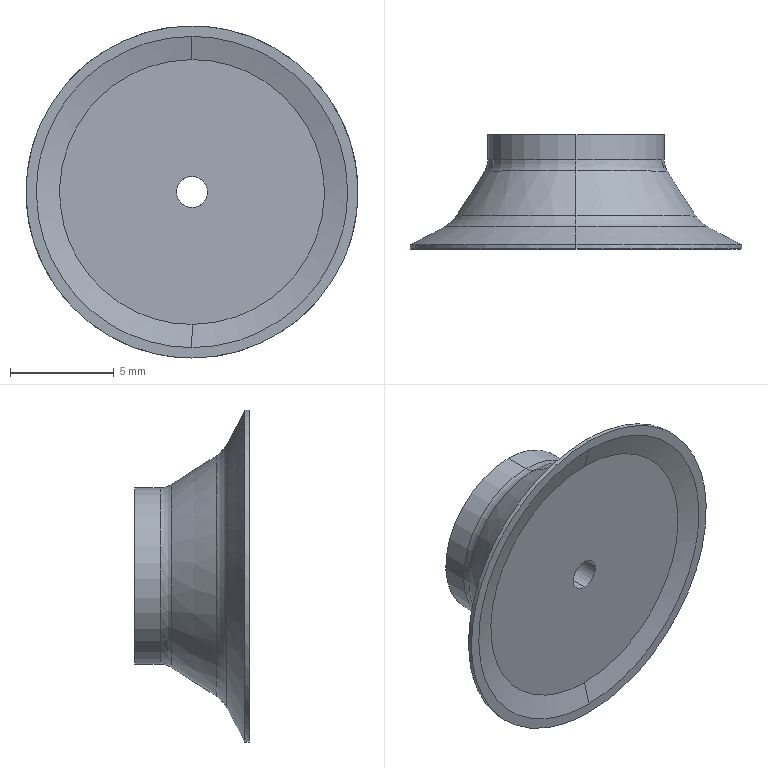Part | SolidWorks | features BaseBody 1 | 1 solid | 25 faces | box 16 x 5.5 x 16 mm | volume 386.03 mm3 | cylinder 10 | cone 6 | plane 5 | torus 4 | commonest cylinder face diameters 1.5 x2 4.2 x2 6 x2 8.5 x2 16 x2
STEP:
#1=CARTESIAN_POINT('',(0.,3.5,3.));
#2=VERTEX_POINT('',#1);
#3=CARTESIAN_POINT('',(0.,3.5,-3.));
#4=VERTEX_POINT('',#3);
#5=CARTESIAN_POINT('',(0.,3.5,3.));
#6=CARTESIAN_POINT('',(-0.3978,3.5,3.));
#7=CARTESIAN_POINT('',(-0.7805,3.5,2.924));
#8=CARTESIAN_POINT('',(-1.516,3.5,2.619));
#9=CARTESIAN_POINT('',(-1.84,3.5,2.403));
#10=CARTESIAN_POINT('',(-2.403,3.5,1.84));
#11=CARTESIAN_POINT('',(-2.619,3.5,1.516));
#12=CARTESIAN_POINT('',(-2.924,3.5,0.7805));
#13=CARTESIAN_POINT('',(-3.,3.5,0.3978));
#14=CARTESIAN_POINT('',(-3.,3.5,-0.3978));
#15=CARTESIAN_POINT('',(-2.924,3.5,-0.7805));
#16=CARTESIAN_POINT('',(-2.619,3.5,-1.516));
#17=CARTESIAN_POINT('',(-2.403,3.5,-1.84));
#18=CARTESIAN_POINT('',(-1.84,3.5,-2.403));
#19=CARTESIAN_POINT('',(-1.516,3.5,-2.619));
#20=CARTESIAN_POINT('',(-0.7805,3.5,-2.924));
#21=CARTESIAN_POINT('',(-0.3978,3.5,-3.));
#22=CARTESIAN_POINT('',(0.,3.5,-3.));
#23=B_SPLINE_CURVE_WITH_KNOTS('',3,(#5,#6,#7,#8,#9,#10,#11,#12,#13,#14,#15,#16,#17,#18,#19,#20,#21,#22),.UNSPECIFIED.,.F.,.F.,(4,2,2,2,2,2,2,2,4),(3.142,3.534,3.927,4.32,4.712,5.105,5.498,5.89,6.283),.UNSPECIFIED.);
#24=EDGE_CURVE('',#2,#4,#23,.T.);
#25=ORIENTED_EDGE('',*,*,#24,.F.);
#26=CARTESIAN_POINT('',(0.,1.5,3.));
#27=VERTEX_POINT('',#26);
#28=CARTESIAN_POINT('',(0.,1.5,3.));
#29=DIRECTION('',(0.,-1.,0.));
#30=VECTOR('',#29,1000.);
#31=LINE('',#28,#30);
#32=EDGE_CURVE('',#2,#27,#31,.T.);
#33=ORIENTED_EDGE('',*,*,#32,.T.);
#34=CARTESIAN_POINT('',(0.,1.5,-3.));
#35=VERTEX_POINT('',#34);
#36=CARTESIAN_POINT('',(0.,1.5,3.));
#37=CARTESIAN_POINT('',(-0.3927,1.5,3.));
#38=CARTESIAN_POINT('',(-0.7852,1.5,2.922));
#39=CARTESIAN_POINT('',(-1.511,1.5,2.621));
#40=CARTESIAN_POINT('',(-1.844,1.5,2.399));
#41=CARTESIAN_POINT('',(-2.399,1.5,1.844));
#42=CARTESIAN_POINT('',(-2.621,1.5,1.511));
#43=CARTESIAN_POINT('',(-2.922,1.5,0.7852));
#44=CARTESIAN_POINT('',(-3.,1.5,0.3927));
#45=CARTESIAN_POINT('',(-3.,1.5,-0.3927));
#46=CARTESIAN_POINT('',(-2.922,1.5,-0.7852));
#47=CARTESIAN_POINT('',(-2.621,1.5,-1.511));
#48=CARTESIAN_POINT('',(-2.399,1.5,-1.844));
#49=CARTESIAN_POINT('',(-1.844,1.5,-2.399));
#50=CARTESIAN_POINT('',(-1.511,1.5,-2.621));
#51=CARTESIAN_POINT('',(-0.7852,1.5,-2.922));
#52=CARTESIAN_POINT('',(-0.3927,1.5,-3.));
#53=CARTESIAN_POINT('',(0.,1.5,-3.));
#54=B_SPLINE_CURVE_WITH_KNOTS('',3,(#36,#37,#38,#39,#40,#41,#42,#43,#44,#45,#46,#47,#48,#49,#50,#51,#52,#53),.UNSPECIFIED.,.F.,.F.,(4,2,2,2,2,2,2,2,4),(3.142,3.534,3.927,4.32,4.712,5.105,5.498,5.89,6.283),.UNSPECIFIED.);
#55=EDGE_CURVE('',#27,#35,#54,.T.);
#56=ORIENTED_EDGE('',*,*,#55,.T.);
#57=CARTESIAN_POINT('',(0.,1.5,-3.));
#58=DIRECTION('',(0.,-1.,0.));
#59=VECTOR('',#58,1000.);
#60=LINE('',#57,#59);
#61=EDGE_CURVE('',#4,#35,#60,.T.);
#62=ORIENTED_EDGE('',*,*,#61,.F.);
#63=EDGE_LOOP('',(#25,#33,#56,#62));
#64=FACE_OUTER_BOUND('',#63,.T.);
#65=CARTESIAN_POINT('',(0.,1.5,0.));
#66=DIRECTION('',(0.,-1.,0.));
#67=DIRECTION('',(0.,0.,-1.));
#68=AXIS2_PLACEMENT_3D('',#65,#66,#67);
#69=CYLINDRICAL_SURFACE('',#68,3.);
#70=ADVANCED_FACE('',(#64),#69,.F.);
#71=CARTESIAN_POINT('',(0.,5.5,2.1));
#72=VERTEX_POINT('',#71);
#73=CARTESIAN_POINT('',(0.,5.5,-2.1));
#74=VERTEX_POINT('',#73);
#75=CARTESIAN_POINT('',(0.,5.5,2.1));
#76=CARTESIAN_POINT('',(-0.2785,5.5,2.1));
#77=CARTESIAN_POINT('',(-0.5464,5.5,2.047));
#78=CARTESIAN_POINT('',(-1.061,5.5,1.834));
#79=CARTESIAN_POINT('',(-1.288,5.5,1.682));
#80=CARTESIAN_POINT('',(-1.682,5.5,1.288));
#81=CARTESIAN_POINT('',(-1.834,5.5,1.061));
#82=CARTESIAN_POINT('',(-2.047,5.5,0.5464));
#83=CARTESIAN_POINT('',(-2.1,5.5,0.2785));
#84=CARTESIAN_POINT('',(-2.1,5.5,-0.2785));
#85=CARTESIAN_POINT('',(-2.047,5.5,-0.5464));
#86=CARTESIAN_POINT('',(-1.834,5.5,-1.061));
#87=CARTESIAN_POINT('',(-1.682,5.5,-1.288));
#88=CARTESIAN_POINT('',(-1.288,5.5,-1.682));
#89=CARTESIAN_POINT('',(-1.061,5.5,-1.834));
#90=CARTESIAN_POINT('',(-0.5464,5.5,-2.047));
#91=CARTESIAN_POINT('',(-0.2785,5.5,-2.1));
#92=CARTESIAN_POINT('',(0.,5.5,-2.1));
#93=B_SPLINE_CURVE_WITH_KNOTS('',3,(#75,#76,#77,#78,#79,#80,#81,#82,#83,#84,#85,#86,#87,#88,#89,#90,#91,#92),.UNSPECIFIED.,.F.,.F.,(4,2,2,2,2,2,2,2,4),(3.142,3.534,3.927,4.32,4.712,5.105,5.498,5.89,6.283),.UNSPECIFIED.);
#94=EDGE_CURVE('',#72,#74,#93,.T.);
#95=ORIENTED_EDGE('',*,*,#94,.F.);
#96=CARTESIAN_POINT('',(0.,3.5,2.1));
#97=VERTEX_POINT('',#96);
#98=CARTESIAN_POINT('',(0.,1.5,2.1));
#99=DIRECTION('',(0.,-1.,0.));
#100=VECTOR('',#99,1000.);
#101=LINE('',#98,#100);
#102=EDGE_CURVE('',#72,#97,#101,.T.);
#103=ORIENTED_EDGE('',*,*,#102,.T.);
#104=CARTESIAN_POINT('',(0.,3.5,-2.1));
#105=VERTEX_POINT('',#104);
#106=CARTESIAN_POINT('',(0.,3.5,2.1));
#107=CARTESIAN_POINT('',(-0.2749,3.5,2.1));
#108=CARTESIAN_POINT('',(-0.5497,3.5,2.045));
#109=CARTESIAN_POINT('',(-1.058,3.5,1.835));
#110=CARTESIAN_POINT('',(-1.291,3.5,1.679));
#111=CARTESIAN_POINT('',(-1.679,3.5,1.291));
#112=CARTESIAN_POINT('',(-1.835,3.5,1.058));
#113=CARTESIAN_POINT('',(-2.045,3.5,0.5497));
#114=CARTESIAN_POINT('',(-2.1,3.5,0.2749));
#115=CARTESIAN_POINT('',(-2.1,3.5,-0.2749));
#116=CARTESIAN_POINT('',(-2.045,3.5,-0.5497));
#117=CARTESIAN_POINT('',(-1.835,3.5,-1.058));
#118=CARTESIAN_POINT('',(-1.679,3.5,-1.291));
#119=CARTESIAN_POINT('',(-1.291,3.5,-1.679));
#120=CARTESIAN_POINT('',(-1.058,3.5,-1.835));
#121=CARTESIAN_POINT('',(-0.5497,3.5,-2.045));
#122=CARTESIAN_POINT('',(-0.2749,3.5,-2.1));
#123=CARTESIAN_POINT('',(0.,3.5,-2.1));
#124=B_SPLINE_CURVE_WITH_KNOTS('',3,(#106,#107,#108,#109,#110,#111,#112,#113,#114,#115,#116,#117,#118,#119,#120,#121,#122,#123),.UNSPECIFIED.,.F.,.F.,(4,2,2,2,2,2,2,2,4),(3.142,3.534,3.927,4.32,4.712,5.105,5.498,5.89,6.283),.UNSPECIFIED.);
#125=EDGE_CURVE('',#97,#105,#124,.T.);
#126=ORIENTED_EDGE('',*,*,#125,.T.);
#127=CARTESIAN_POINT('',(0.,1.5,-2.1));
#128=DIRECTION('',(0.,-1.,0.));
#129=VECTOR('',#128,1000.);
#130=LINE('',#127,#129);
#131=EDGE_CURVE('',#74,#105,#130,.T.);
#132=ORIENTED_EDGE('',*,*,#131,.F.);
#133=EDGE_LOOP('',(#95,#103,#126,#132));
#134=FACE_OUTER_BOUND('',#133,.T.);
#135=CARTESIAN_POINT('',(0.,1.5,0.));
#136=DIRECTION('',(0.,-1.,0.));
#137=DIRECTION('',(0.,0.,-1.));
#138=AXIS2_PLACEMENT_3D('',#135,#136,#137);
#139=CYLINDRICAL_SURFACE('',#138,2.1);
#140=ADVANCED_FACE('',(#134),#139,.F.);
#141=CARTESIAN_POINT('',(0.,5.5,-4.25));
#142=VERTEX_POINT('',#141);
#143=CARTESIAN_POINT('',(0.,5.5,4.25));
#144=VERTEX_POINT('',#143);
#145=CARTESIAN_POINT('',(0.,5.5,-4.25));
#146=CARTESIAN_POINT('',(0.5563,5.5,-4.25));
#147=CARTESIAN_POINT('',(1.112,5.5,-4.139));
#148=CARTESIAN_POINT('',(2.14,5.5,-3.714));
#149=CARTESIAN_POINT('',(2.612,5.5,-3.399));
#150=CARTESIAN_POINT('',(3.399,5.5,-2.612));
#151=CARTESIAN_POINT('',(3.714,5.5,-2.14));
#152=CARTESIAN_POINT('',(4.139,5.5,-1.112));
#153=CARTESIAN_POINT('',(4.25,5.5,-0.5563));
#154=CARTESIAN_POINT('',(4.25,5.5,0.5563));
#155=CARTESIAN_POINT('',(4.139,5.5,1.112));
#156=CARTESIAN_POINT('',(3.714,5.5,2.14));
#157=CARTESIAN_POINT('',(3.399,5.5,2.612));
#158=CARTESIAN_POINT('',(2.612,5.5,3.399));
#159=CARTESIAN_POINT('',(2.14,5.5,3.714));
#160=CARTESIAN_POINT('',(1.112,5.5,4.139));
#161=CARTESIAN_POINT('',(0.5563,5.5,4.25));
#162=CARTESIAN_POINT('',(0.,5.5,4.25));
#163=B_SPLINE_CURVE_WITH_KNOTS('',3,(#145,#146,#147,#148,#149,#150,#151,#152,#153,#154,#155,#156,#157,#158,#159,#160,#161,#162),.UNSPECIFIED.,.F.,.F.,(4,2,2,2,2,2,2,2,4),(0.,0.3927,0.7854,1.178,1.571,1.963,2.356,2.749,3.142),.UNSPECIFIED.);
#164=EDGE_CURVE('',#142,#144,#163,.T.);
#165=ORIENTED_EDGE('',*,*,#164,.T.);
#166=CARTESIAN_POINT('',(0.,4.291,4.25));
#167=VERTEX_POINT('',#166);
#168=CARTESIAN_POINT('',(0.,0.,4.25));
#169=DIRECTION('',(0.,-1.,0.));
#170=VECTOR('',#169,1000.);
#171=LINE('',#168,#170);
#172=EDGE_CURVE('',#144,#167,#171,.T.);
#173=ORIENTED_EDGE('',*,*,#172,.T.);
#174=CARTESIAN_POINT('',(0.,4.291,-4.25));
#175=VERTEX_POINT('',#174);
#176=CARTESIAN_POINT('',(0.,4.291,-4.25));
#177=CARTESIAN_POINT('',(0.5563,4.291,-4.25));
#178=CARTESIAN_POINT('',(1.112,4.291,-4.139));
#179=CARTESIAN_POINT('',(2.14,4.291,-3.714));
#180=CARTESIAN_POINT('',(2.612,4.291,-3.399));
#181=CARTESIAN_POINT('',(3.399,4.291,-2.612));
#182=CARTESIAN_POINT('',(3.714,4.291,-2.14));
#183=CARTESIAN_POINT('',(4.139,4.291,-1.112));
#184=CARTESIAN_POINT('',(4.25,4.291,-0.5563));
#185=CARTESIAN_POINT('',(4.25,4.291,0.5563));
#186=CARTESIAN_POINT('',(4.139,4.291,1.112));
#187=CARTESIAN_POINT('',(3.714,4.291,2.14));
#188=CARTESIAN_POINT('',(3.399,4.291,2.612));
#189=CARTESIAN_POINT('',(2.612,4.291,3.399));
#190=CARTESIAN_POINT('',(2.14,4.291,3.714));
#191=CARTESIAN_POINT('',(1.112,4.291,4.139));
#192=CARTESIAN_POINT('',(0.5563,4.291,4.25));
#193=CARTESIAN_POINT('',(0.,4.291,4.25));
#194=B_SPLINE_CURVE_WITH_KNOTS('',3,(#176,#177,#178,#179,#180,#181,#182,#183,#184,#185,#186,#187,#188,#189,#190,#191,#192,#193),.UNSPECIFIED.,.F.,.F.,(4,2,2,2,2,2,2,2,4),(0.,0.3927,0.7854,1.178,1.571,1.963,2.356,2.749,3.142),.UNSPECIFIED.);
#195=EDGE_CURVE('',#175,#167,#194,.T.);
#196=ORIENTED_EDGE('',*,*,#195,.F.);
#197=CARTESIAN_POINT('',(0.,0.,-4.25));
#198=DIRECTION('',(0.,-1.,0.));
#199=VECTOR('',#198,1000.);
#200=LINE('',#197,#199);
#201=EDGE_CURVE('',#142,#175,#200,.T.);
#202=ORIENTED_EDGE('',*,*,#201,.F.);
#203=EDGE_LOOP('',(#165,#173,#196,#202));
#204=FACE_OUTER_BOUND('',#203,.T.);
#205=CARTESIAN_POINT('',(0.,0.,0.));
#206=DIRECTION('',(0.,-1.,0.));
#207=DIRECTION('',(0.,0.,-1.));
#208=AXIS2_PLACEMENT_3D('',#205,#206,#207);
#209=CYLINDRICAL_SURFACE('',#208,4.25);
#210=ADVANCED_FACE('',(#204),#209,.T.);
#211=CARTESIAN_POINT('',(0.,3.754,4.406));
#212=VERTEX_POINT('',#211);
#213=CARTESIAN_POINT('',(0.,3.754,-4.406));
#214=VERTEX_POINT('',#213);
#215=CARTESIAN_POINT('',(0.,3.754,4.406));
#216=CARTESIAN_POINT('',(-0.5768,3.754,4.406));
#217=CARTESIAN_POINT('',(-1.153,3.754,4.292));
#218=CARTESIAN_POINT('',(-2.219,3.754,3.85));
#219=CARTESIAN_POINT('',(-2.708,3.754,3.524));
#220=CARTESIAN_POINT('',(-3.524,3.754,2.708));
#221=CARTESIAN_POINT('',(-3.85,3.754,2.219));
#222=CARTESIAN_POINT('',(-4.292,3.754,1.153));
#223=CARTESIAN_POINT('',(-4.406,3.754,0.5768));
#224=CARTESIAN_POINT('',(-4.406,3.754,-0.5768));
#225=CARTESIAN_POINT('',(-4.292,3.754,-1.153));
#226=CARTESIAN_POINT('',(-3.85,3.754,-2.219));
#227=CARTESIAN_POINT('',(-3.524,3.754,-2.708));
#228=CARTESIAN_POINT('',(-2.708,3.754,-3.524));
#229=CARTESIAN_POINT('',(-2.219,3.754,-3.85));
#230=CARTESIAN_POINT('',(-1.153,3.754,-4.292));
#231=CARTESIAN_POINT('',(-0.5768,3.754,-4.406));
#232=CARTESIAN_POINT('',(0.,3.754,-4.406));
#233=B_SPLINE_CURVE_WITH_KNOTS('',3,(#215,#216,#217,#218,#219,#220,#221,#222,#223,#224,#225,#226,#227,#228,#229,#230,#231,#232),.UNSPECIFIED.,.F.,.F.,(4,2,2,2,2,2,2,2,4),(3.142,3.534,3.927,4.32,4.712,5.105,5.498,5.89,6.283),.UNSPECIFIED.);
#234=EDGE_CURVE('',#212,#214,#233,.T.);
#235=ORIENTED_EDGE('',*,*,#234,.F.);
#236=CARTESIAN_POINT('',(0.,4.291,5.25));
#237=DIRECTION('',(1.,0.,0.));
#238=DIRECTION('',(0.,0.,-1.));
#239=AXIS2_PLACEMENT_3D('',#236,#237,#238);
#240=CIRCLE('',#239,1.);
#241=EDGE_CURVE('',#212,#167,#240,.T.);
#242=ORIENTED_EDGE('',*,*,#241,.T.);
#243=CARTESIAN_POINT('',(0.,4.291,4.25));
#244=CARTESIAN_POINT('',(-0.5563,4.291,4.25));
#245=CARTESIAN_POINT('',(-1.112,4.291,4.139));
#246=CARTESIAN_POINT('',(-2.14,4.291,3.714));
#247=CARTESIAN_POINT('',(-2.612,4.291,3.399));
#248=CARTESIAN_POINT('',(-3.399,4.291,2.612));
#249=CARTESIAN_POINT('',(-3.714,4.291,2.14));
#250=CARTESIAN_POINT('',(-4.139,4.291,1.112));
#251=CARTESIAN_POINT('',(-4.25,4.291,0.5563));
#252=CARTESIAN_POINT('',(-4.25,4.291,-0.5563));
#253=CARTESIAN_POINT('',(-4.139,4.291,-1.112));
#254=CARTESIAN_POINT('',(-3.714,4.291,-2.14));
#255=CARTESIAN_POINT('',(-3.399,4.291,-2.612));
#256=CARTESIAN_POINT('',(-2.612,4.291,-3.399));
#257=CARTESIAN_POINT('',(-2.14,4.291,-3.714));
#258=CARTESIAN_POINT('',(-1.112,4.291,-4.139));
#259=CARTESIAN_POINT('',(-0.5563,4.291,-4.25));
#260=CARTESIAN_POINT('',(0.,4.291,-4.25));
#261=B_SPLINE_CURVE_WITH_KNOTS('',3,(#243,#244,#245,#246,#247,#248,#249,#250,#251,#252,#253,#254,#255,#256,#257,#258,#259,#260),.UNSPECIFIED.,.F.,.F.,(4,2,2,2,2,2,2,2,4),(3.142,3.534,3.927,4.32,4.712,5.105,5.498,5.89,6.283),.UNSPECIFIED.);
#262=EDGE_CURVE('',#167,#175,#261,.T.);
#263=ORIENTED_EDGE('',*,*,#262,.T.);
#264=CARTESIAN_POINT('',(0.,4.291,-5.25));
#265=DIRECTION('',(-1.,0.,0.));
#266=DIRECTION('',(0.,0.,1.));
#267=AXIS2_PLACEMENT_3D('',#264,#265,#266);
#268=CIRCLE('',#267,1.);
#269=EDGE_CURVE('',#214,#175,#268,.T.);
#270=ORIENTED_EDGE('',*,*,#269,.F.);
#271=EDGE_LOOP('',(#235,#242,#263,#270));
#272=FACE_OUTER_BOUND('',#271,.T.);
#273=CARTESIAN_POINT('',(0.,4.291,0.));
#274=DIRECTION('',(0.,-1.,0.));
#275=DIRECTION('',(0.,0.,-1.));
#276=AXIS2_PLACEMENT_3D('',#273,#274,#275);
#277=TOROIDAL_SURFACE('',#276,5.25,1.);
#278=ADVANCED_FACE('',(#272),#277,.F.);
#279=CARTESIAN_POINT('',(0.,3.754,-4.406));
#280=CARTESIAN_POINT('',(0.5768,3.754,-4.406));
#281=CARTESIAN_POINT('',(1.153,3.754,-4.292));
#282=CARTESIAN_POINT('',(2.219,3.754,-3.85));
#283=CARTESIAN_POINT('',(2.708,3.754,-3.524));
#284=CARTESIAN_POINT('',(3.524,3.754,-2.708));
#285=CARTESIAN_POINT('',(3.85,3.754,-2.219));
#286=CARTESIAN_POINT('',(4.292,3.754,-1.153));
#287=CARTESIAN_POINT('',(4.406,3.754,-0.5768));
#288=CARTESIAN_POINT('',(4.406,3.754,0.5768));
#289=CARTESIAN_POINT('',(4.292,3.754,1.153));
#290=CARTESIAN_POINT('',(3.85,3.754,2.219));
#291=CARTESIAN_POINT('',(3.524,3.754,2.708));
#292=CARTESIAN_POINT('',(2.708,3.754,3.524));
#293=CARTESIAN_POINT('',(2.219,3.754,3.85));
#294=CARTESIAN_POINT('',(1.153,3.754,4.292));
#295=CARTESIAN_POINT('',(0.5768,3.754,4.406));
#296=CARTESIAN_POINT('',(0.,3.754,4.406));
#297=B_SPLINE_CURVE_WITH_KNOTS('',3,(#279,#280,#281,#282,#283,#284,#285,#286,#287,#288,#289,#290,#291,#292,#293,#294,#295,#296),.UNSPECIFIED.,.F.,.F.,(4,2,2,2,2,2,2,2,4),(0.,0.3927,0.7854,1.178,1.571,1.963,2.356,2.749,3.142),.UNSPECIFIED.);
#298=EDGE_CURVE('',#214,#212,#297,.T.);
#299=ORIENTED_EDGE('',*,*,#298,.T.);
#300=CARTESIAN_POINT('',(0.,1.587,5.786));
#301=VERTEX_POINT('',#300);
#302=CARTESIAN_POINT('',(0.,1.587,5.786));
#303=DIRECTION('',(0.,-0.8437,0.5369));
#304=VECTOR('',#303,1000.);
#305=LINE('',#302,#304);
#306=EDGE_CURVE('',#212,#301,#305,.T.);
#307=ORIENTED_EDGE('',*,*,#306,.T.);
#308=CARTESIAN_POINT('',(0.,1.587,-5.786));
#309=VERTEX_POINT('',#308);
#310=CARTESIAN_POINT('',(0.,1.587,-5.786));
#311=CARTESIAN_POINT('',(0.7573,1.587,-5.786));
#312=CARTESIAN_POINT('',(1.514,1.587,-5.635));
#313=CARTESIAN_POINT('',(2.914,1.587,-5.055));
#314=CARTESIAN_POINT('',(3.555,1.587,-4.626));
#315=CARTESIAN_POINT('',(4.626,1.587,-3.555));
#316=CARTESIAN_POINT('',(5.055,1.587,-2.914));
#317=CARTESIAN_POINT('',(5.635,1.587,-1.514));
#318=CARTESIAN_POINT('',(5.786,1.587,-0.7573));
#319=CARTESIAN_POINT('',(5.786,1.587,0.7573));
#320=CARTESIAN_POINT('',(5.635,1.587,1.514));
#321=CARTESIAN_POINT('',(5.055,1.587,2.914));
#322=CARTESIAN_POINT('',(4.626,1.587,3.555));
#323=CARTESIAN_POINT('',(3.555,1.587,4.626));
#324=CARTESIAN_POINT('',(2.914,1.587,5.055));
#325=CARTESIAN_POINT('',(1.514,1.587,5.635));
#326=CARTESIAN_POINT('',(0.7573,1.587,5.786));
#327=CARTESIAN_POINT('',(0.,1.587,5.786));
#328=B_SPLINE_CURVE_WITH_KNOTS('',3,(#310,#311,#312,#313,#314,#315,#316,#317,#318,#319,#320,#321,#322,#323,#324,#325,#326,#327),.UNSPECIFIED.,.F.,.F.,(4,2,2,2,2,2,2,2,4),(0.,0.3927,0.7854,1.178,1.571,1.963,2.356,2.749,3.142),.UNSPECIFIED.);
#329=EDGE_CURVE('',#309,#301,#328,.T.);
#330=ORIENTED_EDGE('',*,*,#329,.F.);
#331=CARTESIAN_POINT('',(0.,1.587,-5.786));
#332=DIRECTION('',(0.,-0.8437,-0.5369));
#333=VECTOR('',#332,1000.);
#334=LINE('',#331,#333);
#335=EDGE_CURVE('',#214,#309,#334,.T.);
#336=ORIENTED_EDGE('',*,*,#335,.F.);
#337=EDGE_LOOP('',(#299,#307,#330,#336));
#338=FACE_OUTER_BOUND('',#337,.T.);
#339=CARTESIAN_POINT('',(0.,1.587,0.));
#340=DIRECTION('',(0.,-1.,0.));
#341=DIRECTION('',(0.,0.,-1.));
#342=AXIS2_PLACEMENT_3D('',#339,#340,#341);
#343=CONICAL_SURFACE('',#342,5.786,0.5667);
#344=ADVANCED_FACE('',(#338),#343,.T.);
#345=CARTESIAN_POINT('',(0.,1.064,6.354));
#346=VERTEX_POINT('',#345);
#347=CARTESIAN_POINT('',(0.,1.064,-6.354));
#348=VERTEX_POINT('',#347);
#349=CARTESIAN_POINT('',(0.,1.064,6.354));
#350=CARTESIAN_POINT('',(-0.8317,1.064,6.354));
#351=CARTESIAN_POINT('',(-1.663,1.064,6.188));
#352=CARTESIAN_POINT('',(-3.2,1.064,5.552));
#353=CARTESIAN_POINT('',(-3.905,1.064,5.081));
#354=CARTESIAN_POINT('',(-5.081,1.064,3.905));
#355=CARTESIAN_POINT('',(-5.552,1.064,3.2));
#356=CARTESIAN_POINT('',(-6.188,1.064,1.663));
#357=CARTESIAN_POINT('',(-6.354,1.064,0.8317));
#358=CARTESIAN_POINT('',(-6.354,1.064,-0.8317));
#359=CARTESIAN_POINT('',(-6.188,1.064,-1.663));
#360=CARTESIAN_POINT('',(-5.552,1.064,-3.2));
#361=CARTESIAN_POINT('',(-5.081,1.064,-3.905));
#362=CARTESIAN_POINT('',(-3.905,1.064,-5.081));
#363=CARTESIAN_POINT('',(-3.2,1.064,-5.552));
#364=CARTESIAN_POINT('',(-1.663,1.064,-6.188));
#365=CARTESIAN_POINT('',(-0.8317,1.064,-6.354));
#366=CARTESIAN_POINT('',(0.,1.064,-6.354));
#367=B_SPLINE_CURVE_WITH_KNOTS('',3,(#349,#350,#351,#352,#353,#354,#355,#356,#357,#358,#359,#360,#361,#362,#363,#364,#365,#366),.UNSPECIFIED.,.F.,.F.,(4,2,2,2,2,2,2,2,4),(3.142,3.534,3.927,4.32,4.712,5.105,5.498,5.89,6.283),.UNSPECIFIED.);
#368=EDGE_CURVE('',#346,#348,#367,.T.);
#369=ORIENTED_EDGE('',*,*,#368,.F.);
#370=CARTESIAN_POINT('',(0.,2.392,7.051));
#371=DIRECTION('',(1.,0.,0.));
#372=DIRECTION('',(0.,0.,-1.));
#373=AXIS2_PLACEMENT_3D('',#370,#371,#372);
#374=CIRCLE('',#373,1.5);
#375=EDGE_CURVE('',#346,#301,#374,.T.);
#376=ORIENTED_EDGE('',*,*,#375,.T.);
#377=CARTESIAN_POINT('',(0.,1.587,5.786));
#378=CARTESIAN_POINT('',(-0.7573,1.587,5.786));
#379=CARTESIAN_POINT('',(-1.514,1.587,5.635));
#380=CARTESIAN_POINT('',(-2.914,1.587,5.055));
#381=CARTESIAN_POINT('',(-3.555,1.587,4.626));
#382=CARTESIAN_POINT('',(-4.626,1.587,3.555));
#383=CARTESIAN_POINT('',(-5.055,1.587,2.914));
#384=CARTESIAN_POINT('',(-5.635,1.587,1.514));
#385=CARTESIAN_POINT('',(-5.786,1.587,0.7573));
#386=CARTESIAN_POINT('',(-5.786,1.587,-0.7573));
#387=CARTESIAN_POINT('',(-5.635,1.587,-1.514));
#388=CARTESIAN_POINT('',(-5.055,1.587,-2.914));
#389=CARTESIAN_POINT('',(-4.626,1.587,-3.555));
#390=CARTESIAN_POINT('',(-3.555,1.587,-4.626));
#391=CARTESIAN_POINT('',(-2.914,1.587,-5.055));
#392=CARTESIAN_POINT('',(-1.514,1.587,-5.635));
#393=CARTESIAN_POINT('',(-0.7573,1.587,-5.786));
#394=CARTESIAN_POINT('',(0.,1.587,-5.786));
#395=B_SPLINE_CURVE_WITH_KNOTS('',3,(#377,#378,#379,#380,#381,#382,#383,#384,#385,#386,#387,#388,#389,#390,#391,#392,#393,#394),.UNSPECIFIED.,.F.,.F.,(4,2,2,2,2,2,2,2,4),(3.142,3.534,3.927,4.32,4.712,5.105,5.498,5.89,6.283),.UNSPECIFIED.);
#396=EDGE_CURVE('',#301,#309,#395,.T.);
#397=ORIENTED_EDGE('',*,*,#396,.T.);
#398=CARTESIAN_POINT('',(0.,2.392,-7.051));
#399=DIRECTION('',(-1.,0.,0.));
#400=DIRECTION('',(0.,0.,1.));
#401=AXIS2_PLACEMENT_3D('',#398,#399,#400);
#402=CIRCLE('',#401,1.5);
#403=EDGE_CURVE('',#348,#309,#402,.T.);
#404=ORIENTED_EDGE('',*,*,#403,.F.);
#405=EDGE_LOOP('',(#369,#376,#397,#404));
#406=FACE_OUTER_BOUND('',#405,.T.);
#407=CARTESIAN_POINT('',(0.,2.392,0.));
#408=DIRECTION('',(0.,-1.,0.));
#409=DIRECTION('',(0.,0.,-1.));
#410=AXIS2_PLACEMENT_3D('',#407,#408,#409);
#411=TOROIDAL_SURFACE('',#410,7.051,1.5);
#412=ADVANCED_FACE('',(#406),#411,.F.);
#413=CARTESIAN_POINT('',(0.,1.064,-6.354));
#414=CARTESIAN_POINT('',(0.8317,1.064,-6.354));
#415=CARTESIAN_POINT('',(1.663,1.064,-6.188));
#416=CARTESIAN_POINT('',(3.2,1.064,-5.552));
#417=CARTESIAN_POINT('',(3.905,1.064,-5.081));
#418=CARTESIAN_POINT('',(5.081,1.064,-3.905));
#419=CARTESIAN_POINT('',(5.552,1.064,-3.2));
#420=CARTESIAN_POINT('',(6.188,1.064,-1.663));
#421=CARTESIAN_POINT('',(6.354,1.064,-0.8317));
#422=CARTESIAN_POINT('',(6.354,1.064,0.8317));
#423=CARTESIAN_POINT('',(6.188,1.064,1.663));
#424=CARTESIAN_POINT('',(5.552,1.064,3.2));
#425=CARTESIAN_POINT('',(5.081,1.064,3.905));
#426=CARTESIAN_POINT('',(3.905,1.064,5.081));
#427=CARTESIAN_POINT('',(3.2,1.064,5.552));
#428=CARTESIAN_POINT('',(1.663,1.064,6.188));
#429=CARTESIAN_POINT('',(0.8317,1.064,6.354));
#430=CARTESIAN_POINT('',(0.,1.064,6.354));
#431=B_SPLINE_CURVE_WITH_KNOTS('',3,(#413,#414,#415,#416,#417,#418,#419,#420,#421,#422,#423,#424,#425,#426,#427,#428,#429,#430),.UNSPECIFIED.,.F.,.F.,(4,2,2,2,2,2,2,2,4),(0.,0.3927,0.7854,1.178,1.571,1.963,2.356,2.749,3.142),.UNSPECIFIED.);
#432=EDGE_CURVE('',#348,#346,#431,.T.);
#433=ORIENTED_EDGE('',*,*,#432,.T.);
#434=CARTESIAN_POINT('',(0.,0.2,8.));
#435=VERTEX_POINT('',#434);
#436=CARTESIAN_POINT('',(0.,0.2,8.));
#437=DIRECTION('',(0.,-0.4648,0.8854));
#438=VECTOR('',#437,1000.);
#439=LINE('',#436,#438);
#440=EDGE_CURVE('',#346,#435,#439,.T.);
#441=ORIENTED_EDGE('',*,*,#440,.T.);
#442=CARTESIAN_POINT('',(0.,0.2,-8.));
#443=VERTEX_POINT('',#442);
#444=CARTESIAN_POINT('',(0.,0.2,-8.));
#445=CARTESIAN_POINT('',(1.047,0.2,-8.));
#446=CARTESIAN_POINT('',(2.094,0.2,-7.792));
#447=CARTESIAN_POINT('',(4.029,0.2,-6.99));
#448=CARTESIAN_POINT('',(4.916,0.2,-6.397));
#449=CARTESIAN_POINT('',(6.397,0.2,-4.916));
#450=CARTESIAN_POINT('',(6.99,0.2,-4.029));
#451=CARTESIAN_POINT('',(7.792,0.2,-2.094));
#452=CARTESIAN_POINT('',(8.,0.2,-1.047));
#453=CARTESIAN_POINT('',(8.,0.2,1.047));
#454=CARTESIAN_POINT('',(7.792,0.2,2.094));
#455=CARTESIAN_POINT('',(6.99,0.2,4.029));
#456=CARTESIAN_POINT('',(6.397,0.2,4.916));
#457=CARTESIAN_POINT('',(4.916,0.2,6.397));
#458=CARTESIAN_POINT('',(4.029,0.2,6.99));
#459=CARTESIAN_POINT('',(2.094,0.2,7.792));
#460=CARTESIAN_POINT('',(1.047,0.2,8.));
#461=CARTESIAN_POINT('',(0.,0.2,8.));
#462=B_SPLINE_CURVE_WITH_KNOTS('',3,(#444,#445,#446,#447,#448,#449,#450,#451,#452,#453,#454,#455,#456,#457,#458,#459,#460,#461),.UNSPECIFIED.,.F.,.F.,(4,2,2,2,2,2,2,2,4),(0.,0.3927,0.7854,1.178,1.571,1.963,2.356,2.749,3.142),.UNSPECIFIED.);
#463=EDGE_CURVE('',#443,#435,#462,.T.);
#464=ORIENTED_EDGE('',*,*,#463,.F.);
#465=CARTESIAN_POINT('',(0.,0.2,-8.));
#466=DIRECTION('',(0.,-0.4648,-0.8854));
#467=VECTOR('',#466,1000.);
#468=LINE('',#465,#467);
#469=EDGE_CURVE('',#348,#443,#468,.T.);
#470=ORIENTED_EDGE('',*,*,#469,.F.);
#471=EDGE_LOOP('',(#433,#441,#464,#470));
#472=FACE_OUTER_BOUND('',#471,.T.);
#473=CARTESIAN_POINT('',(0.,0.2,0.));
#474=DIRECTION('',(0.,-1.,0.));
#475=DIRECTION('',(0.,0.,-1.));
#476=AXIS2_PLACEMENT_3D('',#473,#474,#475);
#477=CONICAL_SURFACE('',#476,8.,1.087);
#478=ADVANCED_FACE('',(#472),#477,.T.);
#479=ORIENTED_EDGE('',*,*,#463,.T.);
#480=CARTESIAN_POINT('',(0.,0.,8.));
#481=VERTEX_POINT('',#480);
#482=CARTESIAN_POINT('',(0.,0.,8.));
#483=DIRECTION('',(0.,-1.,0.));
#484=VECTOR('',#483,1000.);
#485=LINE('',#482,#484);
#486=EDGE_CURVE('',#435,#481,#485,.T.);
#487=ORIENTED_EDGE('',*,*,#486,.T.);
#488=CARTESIAN_POINT('',(0.,0.,-8.));
#489=VERTEX_POINT('',#488);
#490=CARTESIAN_POINT('',(0.,0.,-8.));
#491=CARTESIAN_POINT('',(0.5253,0.,-8.));
#492=CARTESIAN_POINT('',(1.046,0.,-7.949));
#493=CARTESIAN_POINT('',(2.076,0.,-7.744));
#494=CARTESIAN_POINT('',(2.576,0.,-7.592));
#495=CARTESIAN_POINT('',(3.547,0.,-7.19));
#496=CARTESIAN_POINT('',(4.008,0.,-6.944));
#497=CARTESIAN_POINT('',(4.881,0.,-6.36));
#498=CARTESIAN_POINT('',(5.285,0.,-6.028));
#499=CARTESIAN_POINT('',(6.028,0.,-5.285));
#500=CARTESIAN_POINT('',(6.36,0.,-4.881));
#501=CARTESIAN_POINT('',(6.944,0.,-4.008));
#502=CARTESIAN_POINT('',(7.19,0.,-3.547));
#503=CARTESIAN_POINT('',(7.592,0.,-2.576));
#504=CARTESIAN_POINT('',(7.744,0.,-2.076));
#505=CARTESIAN_POINT('',(7.949,0.,-1.046));
#506=CARTESIAN_POINT('',(8.,0.,-0.5253));
#507=CARTESIAN_POINT('',(8.,0.,0.5253));
#508=CARTESIAN_POINT('',(7.949,0.,1.046));
#509=CARTESIAN_POINT('',(7.744,0.,2.076));
#510=CARTESIAN_POINT('',(7.592,0.,2.576));
#511=CARTESIAN_POINT('',(7.19,0.,3.547));
#512=CARTESIAN_POINT('',(6.944,0.,4.008));
#513=CARTESIAN_POINT('',(6.36,0.,4.881));
#514=CARTESIAN_POINT('',(6.028,0.,5.285));
#515=CARTESIAN_POINT('',(5.285,0.,6.028));
#516=CARTESIAN_POINT('',(4.881,0.,6.36));
#517=CARTESIAN_POINT('',(4.008,0.,6.944));
#518=CARTESIAN_POINT('',(3.547,0.,7.19));
#519=CARTESIAN_POINT('',(2.576,0.,7.592));
#520=CARTESIAN_POINT('',(2.076,0.,7.744));
#521=CARTESIAN_POINT('',(1.046,0.,7.949));
#522=CARTESIAN_POINT('',(0.5253,0.,8.));
#523=CARTESIAN_POINT('',(0.,0.,8.));
#524=B_SPLINE_CURVE_WITH_KNOTS('',3,(#490,#491,#492,#493,#494,#495,#496,#497,#498,#499,#500,#501,#502,#503,#504,#505,#506,#507,#508,#509,#510,#511,#512,#513,#514,#515,#516,#517,#518,#519,#520,#521,#522,#523),.UNSPECIFIED.,.F.,.F.,(4,2,2,2,2,2,2,2,2,2,2,2,2,2,2,2,4),(0.,0.1963,0.3927,0.589,0.7854,0.9817,1.178,1.374,1.571,1.767,1.963,2.16,2.356,2.553,2.749,2.945,3.142),.UNSPECIFIED.);
#525=EDGE_CURVE('',#489,#481,#524,.T.);
#526=ORIENTED_EDGE('',*,*,#525,.F.);
#527=CARTESIAN_POINT('',(0.,0.,-8.));
#528=DIRECTION('',(0.,-1.,0.));
#529=VECTOR('',#528,1000.);
#530=LINE('',#527,#529);
#531=EDGE_CURVE('',#443,#489,#530,.T.);
#532=ORIENTED_EDGE('',*,*,#531,.F.);
#533=EDGE_LOOP('',(#479,#487,#526,#532));
#534=FACE_OUTER_BOUND('',#533,.T.);
#535=CARTESIAN_POINT('',(0.,0.,0.));
#536=DIRECTION('',(0.,-1.,0.));
#537=DIRECTION('',(0.,0.,-1.));
#538=AXIS2_PLACEMENT_3D('',#535,#536,#537);
#539=CYLINDRICAL_SURFACE('',#538,8.);
#540=ADVANCED_FACE('',(#534),#539,.T.);
#541=CARTESIAN_POINT('',(0.,0.3,6.38));
#542=VERTEX_POINT('',#541);
#543=CARTESIAN_POINT('',(0.,0.3,-6.38));
#544=VERTEX_POINT('',#543);
#545=CARTESIAN_POINT('',(0.,0.3,6.38));
#546=CARTESIAN_POINT('',(-0.8379,0.3,6.38));
#547=CARTESIAN_POINT('',(-1.668,0.3,6.215));
#548=CARTESIAN_POINT('',(-3.216,0.3,5.574));
#549=CARTESIAN_POINT('',(-3.919,0.3,5.104));
#550=CARTESIAN_POINT('',(-5.104,0.3,3.919));
#551=CARTESIAN_POINT('',(-5.574,0.3,3.216));
#552=CARTESIAN_POINT('',(-6.215,0.3,1.668));
#553=CARTESIAN_POINT('',(-6.38,0.3,0.8379));
#554=CARTESIAN_POINT('',(-6.38,0.3,-0.8379));
#555=CARTESIAN_POINT('',(-6.215,0.3,-1.668));
#556=CARTESIAN_POINT('',(-5.574,0.3,-3.216));
#557=CARTESIAN_POINT('',(-5.104,0.3,-3.919));
#558=CARTESIAN_POINT('',(-3.919,0.3,-5.104));
#559=CARTESIAN_POINT('',(-3.216,0.3,-5.574));
#560=CARTESIAN_POINT('',(-1.668,0.3,-6.215));
#561=CARTESIAN_POINT('',(-0.8379,0.3,-6.38));
#562=CARTESIAN_POINT('',(0.,0.3,-6.38));
#563=B_SPLINE_CURVE_WITH_KNOTS('',3,(#545,#546,#547,#548,#549,#550,#551,#552,#553,#554,#555,#556,#557,#558,#559,#560,#561,#562),.UNSPECIFIED.,.F.,.F.,(4,2,2,2,2,2,2,2,4),(3.142,3.534,3.927,4.32,4.712,5.105,5.498,5.89,6.283),.UNSPECIFIED.);
#564=EDGE_CURVE('',#542,#544,#563,.T.);
#565=ORIENTED_EDGE('',*,*,#564,.F.);
#566=CARTESIAN_POINT('',(0.,0.,7.5));
#567=VERTEX_POINT('',#566);
#568=CARTESIAN_POINT('',(0.,0.3,6.38));
#569=DIRECTION('',(0.,-0.2588,0.9659));
#570=VECTOR('',#569,1000.);
#571=LINE('',#568,#570);
#572=EDGE_CURVE('',#542,#567,#571,.T.);
#573=ORIENTED_EDGE('',*,*,#572,.T.);
#574=CARTESIAN_POINT('',(0.,0.,-7.5));
#575=VERTEX_POINT('',#574);
#576=CARTESIAN_POINT('',(0.,0.,7.5));
#577=CARTESIAN_POINT('',(-0.9817,0.,7.5));
#578=CARTESIAN_POINT('',(-1.963,0.,7.305));
#579=CARTESIAN_POINT('',(-3.777,0.,6.553));
#580=CARTESIAN_POINT('',(-4.609,0.,5.998));
#581=CARTESIAN_POINT('',(-5.998,0.,4.609));
#582=CARTESIAN_POINT('',(-6.553,0.,3.777));
#583=CARTESIAN_POINT('',(-7.305,0.,1.963));
#584=CARTESIAN_POINT('',(-7.5,0.,0.9817));
#585=CARTESIAN_POINT('',(-7.5,0.,-0.9817));
#586=CARTESIAN_POINT('',(-7.305,0.,-1.963));
#587=CARTESIAN_POINT('',(-6.553,0.,-3.777));
#588=CARTESIAN_POINT('',(-5.998,0.,-4.609));
#589=CARTESIAN_POINT('',(-4.609,0.,-5.998));
#590=CARTESIAN_POINT('',(-3.777,0.,-6.553));
#591=CARTESIAN_POINT('',(-1.963,0.,-7.305));
#592=CARTESIAN_POINT('',(-0.9817,0.,-7.5));
#593=CARTESIAN_POINT('',(0.,0.,-7.5));
#594=B_SPLINE_CURVE_WITH_KNOTS('',3,(#576,#577,#578,#579,#580,#581,#582,#583,#584,#585,#586,#587,#588,#589,#590,#591,#592,#593),.UNSPECIFIED.,.F.,.F.,(4,2,2,2,2,2,2,2,4),(3.142,3.534,3.927,4.32,4.712,5.105,5.498,5.89,6.283),.UNSPECIFIED.);
#595=EDGE_CURVE('',#567,#575,#594,.T.);
#596=ORIENTED_EDGE('',*,*,#595,.T.);
#597=CARTESIAN_POINT('',(0.,0.3,-6.38));
#598=DIRECTION('',(0.,-0.2588,-0.9659));
#599=VECTOR('',#598,1000.);
#600=LINE('',#597,#599);
#601=EDGE_CURVE('',#544,#575,#600,.T.);
#602=ORIENTED_EDGE('',*,*,#601,.F.);
#603=EDGE_LOOP('',(#565,#573,#596,#602));
#604=FACE_OUTER_BOUND('',#603,.T.);
#605=CARTESIAN_POINT('',(0.,0.3,0.));
#606=DIRECTION('',(0.,-1.,0.));
#607=DIRECTION('',(0.,0.,-1.));
#608=AXIS2_PLACEMENT_3D('',#605,#606,#607);
#609=CONICAL_SURFACE('',#608,6.38,1.309);
#610=ADVANCED_FACE('',(#604),#609,.F.);
#611=CARTESIAN_POINT('',(0.,1.5,-0.75));
#612=VERTEX_POINT('',#611);
#613=CARTESIAN_POINT('',(0.,1.5,0.75));
#614=VERTEX_POINT('',#613);
#615=CARTESIAN_POINT('',(0.,1.5,-0.75));
#616=CARTESIAN_POINT('',(-0.1963,1.5,-0.75));
#617=CARTESIAN_POINT('',(-0.3915,1.5,-0.6692));
#618=CARTESIAN_POINT('',(-0.6692,1.5,-0.3915));
#619=CARTESIAN_POINT('',(-0.75,1.5,-0.1963));
#620=CARTESIAN_POINT('',(-0.75,1.5,0.1963));
#621=CARTESIAN_POINT('',(-0.6692,1.5,0.3915));
#622=CARTESIAN_POINT('',(-0.3915,1.5,0.6692));
#623=CARTESIAN_POINT('',(-0.1963,1.5,0.75));
#624=CARTESIAN_POINT('',(0.,1.5,0.75));
#625=B_SPLINE_CURVE_WITH_KNOTS('',3,(#615,#616,#617,#618,#619,#620,#621,#622,#623,#624),.UNSPECIFIED.,.F.,.F.,(4,2,2,2,4),(3.142,3.927,4.712,5.498,6.283),.UNSPECIFIED.);
#626=EDGE_CURVE('',#612,#614,#625,.T.);
#627=ORIENTED_EDGE('',*,*,#626,.T.);
#628=CARTESIAN_POINT('',(0.,0.3,0.75));
#629=VERTEX_POINT('',#628);
#630=CARTESIAN_POINT('',(0.,0.,0.75));
#631=DIRECTION('',(0.,-1.,0.));
#632=VECTOR('',#631,1000.);
#633=LINE('',#630,#632);
#634=EDGE_CURVE('',#614,#629,#633,.T.);
#635=ORIENTED_EDGE('',*,*,#634,.T.);
#636=CARTESIAN_POINT('',(0.,0.3,-0.75));
#637=VERTEX_POINT('',#636);
#638=CARTESIAN_POINT('',(0.,0.3,0.75));
#639=CARTESIAN_POINT('',(-0.1963,0.3,0.75));
#640=CARTESIAN_POINT('',(-0.3915,0.3,0.6692));
#641=CARTESIAN_POINT('',(-0.6692,0.3,0.3915));
#642=CARTESIAN_POINT('',(-0.75,0.3,0.1963));
#643=CARTESIAN_POINT('',(-0.75,0.3,-0.1963));
#644=CARTESIAN_POINT('',(-0.6692,0.3,-0.3915));
#645=CARTESIAN_POINT('',(-0.3915,0.3,-0.6692));
#646=CARTESIAN_POINT('',(-0.1963,0.3,-0.75));
#647=CARTESIAN_POINT('',(0.,0.3,-0.75));
#648=B_SPLINE_CURVE_WITH_KNOTS('',3,(#638,#639,#640,#641,#642,#643,#644,#645,#646,#647),.UNSPECIFIED.,.F.,.F.,(4,2,2,2,4),(3.142,3.927,4.712,5.498,6.283),.UNSPECIFIED.);
#649=EDGE_CURVE('',#629,#637,#648,.T.);
#650=ORIENTED_EDGE('',*,*,#649,.T.);
#651=CARTESIAN_POINT('',(0.,0.,-0.75));
#652=DIRECTION('',(0.,-1.,0.));
#653=VECTOR('',#652,1000.);
#654=LINE('',#651,#653);
#655=EDGE_CURVE('',#612,#637,#654,.T.);
#656=ORIENTED_EDGE('',*,*,#655,.F.);
#657=EDGE_LOOP('',(#627,#635,#650,#656));
#658=FACE_OUTER_BOUND('',#657,.T.);
#659=CARTESIAN_POINT('',(0.,0.,0.));
#660=DIRECTION('',(0.,-1.,0.));
#661=DIRECTION('',(0.,0.,-1.));
#662=AXIS2_PLACEMENT_3D('',#659,#660,#661);
#663=CYLINDRICAL_SURFACE('',#662,0.75);
#664=ADVANCED_FACE('',(#658),#663,.F.);
#665=ORIENTED_EDGE('',*,*,#634,.F.);
#666=CARTESIAN_POINT('',(0.,1.5,0.75));
#667=CARTESIAN_POINT('',(0.1963,1.5,0.75));
#668=CARTESIAN_POINT('',(0.3915,1.5,0.6692));
#669=CARTESIAN_POINT('',(0.6692,1.5,0.3915));
#670=CARTESIAN_POINT('',(0.75,1.5,0.1963));
#671=CARTESIAN_POINT('',(0.75,1.5,-0.1963));
#672=CARTESIAN_POINT('',(0.6692,1.5,-0.3915));
#673=CARTESIAN_POINT('',(0.3915,1.5,-0.6692));
#674=CARTESIAN_POINT('',(0.1963,1.5,-0.75));
#675=CARTESIAN_POINT('',(0.,1.5,-0.75));
#676=B_SPLINE_CURVE_WITH_KNOTS('',3,(#666,#667,#668,#669,#670,#671,#672,#673,#674,#675),.UNSPECIFIED.,.F.,.F.,(4,2,2,2,4),(0.,0.7854,1.571,2.356,3.142),.UNSPECIFIED.);
#677=EDGE_CURVE('',#614,#612,#676,.T.);
#678=ORIENTED_EDGE('',*,*,#677,.T.);
#679=ORIENTED_EDGE('',*,*,#655,.T.);
#680=CARTESIAN_POINT('',(0.,0.3,-0.75));
#681=CARTESIAN_POINT('',(0.1963,0.3,-0.75));
#682=CARTESIAN_POINT('',(0.3915,0.3,-0.6692));
#683=CARTESIAN_POINT('',(0.6692,0.3,-0.3915));
#684=CARTESIAN_POINT('',(0.75,0.3,-0.1963));
#685=CARTESIAN_POINT('',(0.75,0.3,0.1963));
#686=CARTESIAN_POINT('',(0.6692,0.3,0.3915));
#687=CARTESIAN_POINT('',(0.3915,0.3,0.6692));
#688=CARTESIAN_POINT('',(0.1963,0.3,0.75));
#689=CARTESIAN_POINT('',(0.,0.3,0.75));
#690=B_SPLINE_CURVE_WITH_KNOTS('',3,(#680,#681,#682,#683,#684,#685,#686,#687,#688,#689),.UNSPECIFIED.,.F.,.F.,(4,2,2,2,4),(0.,0.7854,1.571,2.356,3.142),.UNSPECIFIED.);
#691=EDGE_CURVE('',#637,#629,#690,.T.);
#692=ORIENTED_EDGE('',*,*,#691,.T.);
#693=EDGE_LOOP('',(#665,#678,#679,#692));
#694=FACE_OUTER_BOUND('',#693,.T.);
#695=CARTESIAN_POINT('',(0.,0.,0.));
#696=DIRECTION('',(0.,-1.,0.));
#697=DIRECTION('',(0.,0.,-1.));
#698=AXIS2_PLACEMENT_3D('',#695,#696,#697);
#699=CYLINDRICAL_SURFACE('',#698,0.75);
#700=ADVANCED_FACE('',(#694),#699,.F.);
#701=CARTESIAN_POINT('',(0.,0.3,-6.38));
#702=CARTESIAN_POINT('',(0.8379,0.3,-6.38));
#703=CARTESIAN_POINT('',(1.668,0.3,-6.215));
#704=CARTESIAN_POINT('',(3.216,0.3,-5.574));
#705=CARTESIAN_POINT('',(3.919,0.3,-5.104));
#706=CARTESIAN_POINT('',(5.104,0.3,-3.919));
#707=CARTESIAN_POINT('',(5.574,0.3,-3.216));
#708=CARTESIAN_POINT('',(6.215,0.3,-1.668));
#709=CARTESIAN_POINT('',(6.38,0.3,-0.8379));
#710=CARTESIAN_POINT('',(6.38,0.3,0.8379));
#711=CARTESIAN_POINT('',(6.215,0.3,1.668));
#712=CARTESIAN_POINT('',(5.574,0.3,3.216));
#713=CARTESIAN_POINT('',(5.104,0.3,3.919));
#714=CARTESIAN_POINT('',(3.919,0.3,5.104));
#715=CARTESIAN_POINT('',(3.216,0.3,5.574));
#716=CARTESIAN_POINT('',(1.668,0.3,6.215));
#717=CARTESIAN_POINT('',(0.8379,0.3,6.38));
#718=CARTESIAN_POINT('',(0.,0.3,6.38));
#719=B_SPLINE_CURVE_WITH_KNOTS('',3,(#701,#702,#703,#704,#705,#706,#707,#708,#709,#710,#711,#712,#713,#714,#715,#716,#717,#718),.UNSPECIFIED.,.F.,.F.,(4,2,2,2,2,2,2,2,4),(0.,0.3927,0.7854,1.178,1.571,1.963,2.356,2.749,3.142),.UNSPECIFIED.);
#720=EDGE_CURVE('',#544,#542,#719,.T.);
#721=ORIENTED_EDGE('',*,*,#720,.T.);
#722=ORIENTED_EDGE('',*,*,#564,.T.);
#723=EDGE_LOOP('',(#721,#722));
#724=FACE_OUTER_BOUND('',#723,.T.);
#725=ORIENTED_EDGE('',*,*,#691,.F.);
#726=ORIENTED_EDGE('',*,*,#649,.F.);
#727=EDGE_LOOP('',(#725,#726));
#728=FACE_BOUND('',#727,.T.);
#729=CARTESIAN_POINT('',(0.75,0.3,0.));
#730=DIRECTION('',(0.,-1.,0.));
#731=DIRECTION('',(0.,0.,-1.));
#732=AXIS2_PLACEMENT_3D('',#729,#730,#731);
#733=PLANE('',#732);
#734=ADVANCED_FACE('',(#724,#728),#733,.T.);
#735=ORIENTED_EDGE('',*,*,#572,.F.);
#736=ORIENTED_EDGE('',*,*,#720,.F.);
#737=ORIENTED_EDGE('',*,*,#601,.T.);
#738=CARTESIAN_POINT('',(0.,0.,-7.5));
#739=CARTESIAN_POINT('',(0.9817,0.,-7.5));
#740=CARTESIAN_POINT('',(1.963,0.,-7.305));
#741=CARTESIAN_POINT('',(3.777,0.,-6.553));
#742=CARTESIAN_POINT('',(4.609,0.,-5.998));
#743=CARTESIAN_POINT('',(5.998,0.,-4.609));
#744=CARTESIAN_POINT('',(6.553,0.,-3.777));
#745=CARTESIAN_POINT('',(7.305,0.,-1.963));
#746=CARTESIAN_POINT('',(7.5,0.,-0.9817));
#747=CARTESIAN_POINT('',(7.5,0.,0.9817));
#748=CARTESIAN_POINT('',(7.305,0.,1.963));
#749=CARTESIAN_POINT('',(6.553,0.,3.777));
#750=CARTESIAN_POINT('',(5.998,0.,4.609));
#751=CARTESIAN_POINT('',(4.609,0.,5.998));
#752=CARTESIAN_POINT('',(3.777,0.,6.553));
#753=CARTESIAN_POINT('',(1.963,0.,7.305));
#754=CARTESIAN_POINT('',(0.9817,0.,7.5));
#755=CARTESIAN_POINT('',(0.,0.,7.5));
#756=B_SPLINE_CURVE_WITH_KNOTS('',3,(#738,#739,#740,#741,#742,#743,#744,#745,#746,#747,#748,#749,#750,#751,#752,#753,#754,#755),.UNSPECIFIED.,.F.,.F.,(4,2,2,2,2,2,2,2,4),(0.,0.3927,0.7854,1.178,1.571,1.963,2.356,2.749,3.142),.UNSPECIFIED.);
#757=EDGE_CURVE('',#575,#567,#756,.T.);
#758=ORIENTED_EDGE('',*,*,#757,.T.);
#759=EDGE_LOOP('',(#735,#736,#737,#758));
#760=FACE_OUTER_BOUND('',#759,.T.);
#761=CARTESIAN_POINT('',(0.,0.3,0.));
#762=DIRECTION('',(0.,-1.,0.));
#763=DIRECTION('',(0.,0.,-1.));
#764=AXIS2_PLACEMENT_3D('',#761,#762,#763);
#765=CONICAL_SURFACE('',#764,6.38,1.309);
#766=ADVANCED_FACE('',(#760),#765,.F.);
#767=ORIENTED_EDGE('',*,*,#525,.T.);
#768=CARTESIAN_POINT('',(0.,0.,8.));
#769=CARTESIAN_POINT('',(-0.5253,0.,8.));
#770=CARTESIAN_POINT('',(-1.046,0.,7.949));
#771=CARTESIAN_POINT('',(-2.076,0.,7.744));
#772=CARTESIAN_POINT('',(-2.576,0.,7.592));
#773=CARTESIAN_POINT('',(-3.547,0.,7.19));
#774=CARTESIAN_POINT('',(-4.008,0.,6.944));
#775=CARTESIAN_POINT('',(-4.881,0.,6.36));
#776=CARTESIAN_POINT('',(-5.285,0.,6.028));
#777=CARTESIAN_POINT('',(-6.028,0.,5.285));
#778=CARTESIAN_POINT('',(-6.36,0.,4.881));
#779=CARTESIAN_POINT('',(-6.944,0.,4.008));
#780=CARTESIAN_POINT('',(-7.19,0.,3.547));
#781=CARTESIAN_POINT('',(-7.592,0.,2.576));
#782=CARTESIAN_POINT('',(-7.744,0.,2.076));
#783=CARTESIAN_POINT('',(-7.949,0.,1.046));
#784=CARTESIAN_POINT('',(-8.,0.,0.5253));
#785=CARTESIAN_POINT('',(-8.,0.,-0.5253));
#786=CARTESIAN_POINT('',(-7.949,0.,-1.046));
#787=CARTESIAN_POINT('',(-7.744,0.,-2.076));
#788=CARTESIAN_POINT('',(-7.592,0.,-2.576));
#789=CARTESIAN_POINT('',(-7.19,0.,-3.547));
#790=CARTESIAN_POINT('',(-6.944,0.,-4.008));
#791=CARTESIAN_POINT('',(-6.36,0.,-4.881));
#792=CARTESIAN_POINT('',(-6.028,0.,-5.285));
#793=CARTESIAN_POINT('',(-5.285,0.,-6.028));
#794=CARTESIAN_POINT('',(-4.881,0.,-6.36));
#795=CARTESIAN_POINT('',(-4.008,0.,-6.944));
#796=CARTESIAN_POINT('',(-3.547,0.,-7.19));
#797=CARTESIAN_POINT('',(-2.576,0.,-7.592));
#798=CARTESIAN_POINT('',(-2.076,0.,-7.744));
#799=CARTESIAN_POINT('',(-1.046,0.,-7.949));
#800=CARTESIAN_POINT('',(-0.5253,0.,-8.));
#801=CARTESIAN_POINT('',(0.,0.,-8.));
#802=B_SPLINE_CURVE_WITH_KNOTS('',3,(#768,#769,#770,#771,#772,#773,#774,#775,#776,#777,#778,#779,#780,#781,#782,#783,#784,#785,#786,#787,#788,#789,#790,#791,#792,#793,#794,#795,#796,#797,#798,#799,#800,#801),.UNSPECIFIED.,.F.,.F.,(4,2,2,2,2,2,2,2,2,2,2,2,2,2,2,2,4),(3.142,3.338,3.534,3.731,3.927,4.123,4.32,4.516,4.712,4.909,5.105,5.301,5.498,5.694,5.89,6.087,6.283),.UNSPECIFIED.);
#803=EDGE_CURVE('',#481,#489,#802,.T.);
#804=ORIENTED_EDGE('',*,*,#803,.T.);
#805=EDGE_LOOP('',(#767,#804));
#806=FACE_OUTER_BOUND('',#805,.T.);
#807=ORIENTED_EDGE('',*,*,#757,.F.);
#808=ORIENTED_EDGE('',*,*,#595,.F.);
#809=EDGE_LOOP('',(#807,#808));
#810=FACE_BOUND('',#809,.T.);
#811=CARTESIAN_POINT('',(7.5,0.,0.));
#812=DIRECTION('',(0.,-1.,0.));
#813=DIRECTION('',(0.,0.,-1.));
#814=AXIS2_PLACEMENT_3D('',#811,#812,#813);
#815=PLANE('',#814);
#816=ADVANCED_FACE('',(#806,#810),#815,.T.);
#817=ORIENTED_EDGE('',*,*,#486,.F.);
#818=CARTESIAN_POINT('',(0.,0.2,8.));
#819=CARTESIAN_POINT('',(-1.047,0.2,8.));
#820=CARTESIAN_POINT('',(-2.094,0.2,7.792));
#821=CARTESIAN_POINT('',(-4.029,0.2,6.99));
#822=CARTESIAN_POINT('',(-4.916,0.2,6.397));
#823=CARTESIAN_POINT('',(-6.397,0.2,4.916));
#824=CARTESIAN_POINT('',(-6.99,0.2,4.029));
#825=CARTESIAN_POINT('',(-7.792,0.2,2.094));
#826=CARTESIAN_POINT('',(-8.,0.2,1.047));
#827=CARTESIAN_POINT('',(-8.,0.2,-1.047));
#828=CARTESIAN_POINT('',(-7.792,0.2,-2.094));
#829=CARTESIAN_POINT('',(-6.99,0.2,-4.029));
#830=CARTESIAN_POINT('',(-6.397,0.2,-4.916));
#831=CARTESIAN_POINT('',(-4.916,0.2,-6.397));
#832=CARTESIAN_POINT('',(-4.029,0.2,-6.99));
#833=CARTESIAN_POINT('',(-2.094,0.2,-7.792));
#834=CARTESIAN_POINT('',(-1.047,0.2,-8.));
#835=CARTESIAN_POINT('',(0.,0.2,-8.));
#836=B_SPLINE_CURVE_WITH_KNOTS('',3,(#818,#819,#820,#821,#822,#823,#824,#825,#826,#827,#828,#829,#830,#831,#832,#833,#834,#835),.UNSPECIFIED.,.F.,.F.,(4,2,2,2,2,2,2,2,4),(3.142,3.534,3.927,4.32,4.712,5.105,5.498,5.89,6.283),.UNSPECIFIED.);
#837=EDGE_CURVE('',#435,#443,#836,.T.);
#838=ORIENTED_EDGE('',*,*,#837,.T.);
#839=ORIENTED_EDGE('',*,*,#531,.T.);
#840=ORIENTED_EDGE('',*,*,#803,.F.);
#841=EDGE_LOOP('',(#817,#838,#839,#840));
#842=FACE_OUTER_BOUND('',#841,.T.);
#843=CARTESIAN_POINT('',(0.,0.,0.));
#844=DIRECTION('',(0.,-1.,0.));
#845=DIRECTION('',(0.,0.,-1.));
#846=AXIS2_PLACEMENT_3D('',#843,#844,#845);
#847=CYLINDRICAL_SURFACE('',#846,8.);
#848=ADVANCED_FACE('',(#842),#847,.T.);
#849=ORIENTED_EDGE('',*,*,#440,.F.);
#850=ORIENTED_EDGE('',*,*,#368,.T.);
#851=ORIENTED_EDGE('',*,*,#469,.T.);
#852=ORIENTED_EDGE('',*,*,#837,.F.);
#853=EDGE_LOOP('',(#849,#850,#851,#852));
#854=FACE_OUTER_BOUND('',#853,.T.);
#855=CARTESIAN_POINT('',(0.,0.2,0.));
#856=DIRECTION('',(0.,-1.,0.));
#857=DIRECTION('',(0.,0.,-1.));
#858=AXIS2_PLACEMENT_3D('',#855,#856,#857);
#859=CONICAL_SURFACE('',#858,8.,1.087);
#860=ADVANCED_FACE('',(#854),#859,.T.);
#861=ORIENTED_EDGE('',*,*,#375,.F.);
#862=ORIENTED_EDGE('',*,*,#432,.F.);
#863=ORIENTED_EDGE('',*,*,#403,.T.);
#864=ORIENTED_EDGE('',*,*,#329,.T.);
#865=EDGE_LOOP('',(#861,#862,#863,#864));
#866=FACE_OUTER_BOUND('',#865,.T.);
#867=CARTESIAN_POINT('',(0.,2.392,0.));
#868=DIRECTION('',(0.,-1.,0.));
#869=DIRECTION('',(0.,0.,-1.));
#870=AXIS2_PLACEMENT_3D('',#867,#868,#869);
#871=TOROIDAL_SURFACE('',#870,7.051,1.5);
#872=ADVANCED_FACE('',(#866),#871,.F.);
#873=ORIENTED_EDGE('',*,*,#306,.F.);
#874=ORIENTED_EDGE('',*,*,#234,.T.);
#875=ORIENTED_EDGE('',*,*,#335,.T.);
#876=ORIENTED_EDGE('',*,*,#396,.F.);
#877=EDGE_LOOP('',(#873,#874,#875,#876));
#878=FACE_OUTER_BOUND('',#877,.T.);
#879=CARTESIAN_POINT('',(0.,1.587,0.));
#880=DIRECTION('',(0.,-1.,0.));
#881=DIRECTION('',(0.,0.,-1.));
#882=AXIS2_PLACEMENT_3D('',#879,#880,#881);
#883=CONICAL_SURFACE('',#882,5.786,0.5667);
#884=ADVANCED_FACE('',(#878),#883,.T.);
#885=ORIENTED_EDGE('',*,*,#241,.F.);
#886=ORIENTED_EDGE('',*,*,#298,.F.);
#887=ORIENTED_EDGE('',*,*,#269,.T.);
#888=ORIENTED_EDGE('',*,*,#195,.T.);
#889=EDGE_LOOP('',(#885,#886,#887,#888));
#890=FACE_OUTER_BOUND('',#889,.T.);
#891=CARTESIAN_POINT('',(0.,4.291,0.));
#892=DIRECTION('',(0.,-1.,0.));
#893=DIRECTION('',(0.,0.,-1.));
#894=AXIS2_PLACEMENT_3D('',#891,#892,#893);
#895=TOROIDAL_SURFACE('',#894,5.25,1.);
#896=ADVANCED_FACE('',(#890),#895,.F.);
#897=ORIENTED_EDGE('',*,*,#172,.F.);
#898=CARTESIAN_POINT('',(0.,5.5,4.25));
#899=CARTESIAN_POINT('',(-0.5563,5.5,4.25));
#900=CARTESIAN_POINT('',(-1.112,5.5,4.139));
#901=CARTESIAN_POINT('',(-2.14,5.5,3.714));
#902=CARTESIAN_POINT('',(-2.612,5.5,3.399));
#903=CARTESIAN_POINT('',(-3.399,5.5,2.612));
#904=CARTESIAN_POINT('',(-3.714,5.5,2.14));
#905=CARTESIAN_POINT('',(-4.139,5.5,1.112));
#906=CARTESIAN_POINT('',(-4.25,5.5,0.5563));
#907=CARTESIAN_POINT('',(-4.25,5.5,-0.5563));
#908=CARTESIAN_POINT('',(-4.139,5.5,-1.112));
#909=CARTESIAN_POINT('',(-3.714,5.5,-2.14));
#910=CARTESIAN_POINT('',(-3.399,5.5,-2.612));
#911=CARTESIAN_POINT('',(-2.612,5.5,-3.399));
#912=CARTESIAN_POINT('',(-2.14,5.5,-3.714));
#913=CARTESIAN_POINT('',(-1.112,5.5,-4.139));
#914=CARTESIAN_POINT('',(-0.5563,5.5,-4.25));
#915=CARTESIAN_POINT('',(0.,5.5,-4.25));
#916=B_SPLINE_CURVE_WITH_KNOTS('',3,(#898,#899,#900,#901,#902,#903,#904,#905,#906,#907,#908,#909,#910,#911,#912,#913,#914,#915),.UNSPECIFIED.,.F.,.F.,(4,2,2,2,2,2,2,2,4),(3.142,3.534,3.927,4.32,4.712,5.105,5.498,5.89,6.283),.UNSPECIFIED.);
#917=EDGE_CURVE('',#144,#142,#916,.T.);
#918=ORIENTED_EDGE('',*,*,#917,.T.);
#919=ORIENTED_EDGE('',*,*,#201,.T.);
#920=ORIENTED_EDGE('',*,*,#262,.F.);
#921=EDGE_LOOP('',(#897,#918,#919,#920));
#922=FACE_OUTER_BOUND('',#921,.T.);
#923=CARTESIAN_POINT('',(0.,0.,0.));
#924=DIRECTION('',(0.,-1.,0.));
#925=DIRECTION('',(0.,0.,-1.));
#926=AXIS2_PLACEMENT_3D('',#923,#924,#925);
#927=CYLINDRICAL_SURFACE('',#926,4.25);
#928=ADVANCED_FACE('',(#922),#927,.T.);
#929=CARTESIAN_POINT('',(0.,5.5,-2.1));
#930=CARTESIAN_POINT('',(0.2785,5.5,-2.1));
#931=CARTESIAN_POINT('',(0.5464,5.5,-2.047));
#932=CARTESIAN_POINT('',(1.061,5.5,-1.834));
#933=CARTESIAN_POINT('',(1.288,5.5,-1.682));
#934=CARTESIAN_POINT('',(1.682,5.5,-1.288));
#935=CARTESIAN_POINT('',(1.834,5.5,-1.061));
#936=CARTESIAN_POINT('',(2.047,5.5,-0.5464));
#937=CARTESIAN_POINT('',(2.1,5.5,-0.2785));
#938=CARTESIAN_POINT('',(2.1,5.5,0.2785));
#939=CARTESIAN_POINT('',(2.047,5.5,0.5464));
#940=CARTESIAN_POINT('',(1.834,5.5,1.061));
#941=CARTESIAN_POINT('',(1.682,5.5,1.288));
#942=CARTESIAN_POINT('',(1.288,5.5,1.682));
#943=CARTESIAN_POINT('',(1.061,5.5,1.834));
#944=CARTESIAN_POINT('',(0.5464,5.5,2.047));
#945=CARTESIAN_POINT('',(0.2785,5.5,2.1));
#946=CARTESIAN_POINT('',(0.,5.5,2.1));
#947=B_SPLINE_CURVE_WITH_KNOTS('',3,(#929,#930,#931,#932,#933,#934,#935,#936,#937,#938,#939,#940,#941,#942,#943,#944,#945,#946),.UNSPECIFIED.,.F.,.F.,(4,2,2,2,2,2,2,2,4),(0.,0.3927,0.7854,1.178,1.571,1.963,2.356,2.749,3.142),.UNSPECIFIED.);
#948=EDGE_CURVE('',#74,#72,#947,.T.);
#949=ORIENTED_EDGE('',*,*,#948,.T.);
#950=ORIENTED_EDGE('',*,*,#94,.T.);
#951=EDGE_LOOP('',(#949,#950));
#952=FACE_BOUND('',#951,.T.);
#953=ORIENTED_EDGE('',*,*,#164,.F.);
#954=ORIENTED_EDGE('',*,*,#917,.F.);
#955=EDGE_LOOP('',(#953,#954));
#956=FACE_OUTER_BOUND('',#955,.T.);
#957=CARTESIAN_POINT('',(4.25,5.5,0.));
#958=DIRECTION('',(0.,1.,0.));
#959=DIRECTION('',(0.,0.,1.));
#960=AXIS2_PLACEMENT_3D('',#957,#958,#959);
#961=PLANE('',#960);
#962=ADVANCED_FACE('',(#952,#956),#961,.T.);
#963=ORIENTED_EDGE('',*,*,#102,.F.);
#964=ORIENTED_EDGE('',*,*,#948,.F.);
#965=ORIENTED_EDGE('',*,*,#131,.T.);
#966=CARTESIAN_POINT('',(0.,3.5,-2.1));
#967=CARTESIAN_POINT('',(0.2749,3.5,-2.1));
#968=CARTESIAN_POINT('',(0.5497,3.5,-2.045));
#969=CARTESIAN_POINT('',(1.058,3.5,-1.835));
#970=CARTESIAN_POINT('',(1.291,3.5,-1.679));
#971=CARTESIAN_POINT('',(1.679,3.5,-1.291));
#972=CARTESIAN_POINT('',(1.835,3.5,-1.058));
#973=CARTESIAN_POINT('',(2.045,3.5,-0.5497));
#974=CARTESIAN_POINT('',(2.1,3.5,-0.2749));
#975=CARTESIAN_POINT('',(2.1,3.5,0.2749));
#976=CARTESIAN_POINT('',(2.045,3.5,0.5497));
#977=CARTESIAN_POINT('',(1.835,3.5,1.058));
#978=CARTESIAN_POINT('',(1.679,3.5,1.291));
#979=CARTESIAN_POINT('',(1.291,3.5,1.679));
#980=CARTESIAN_POINT('',(1.058,3.5,1.835));
#981=CARTESIAN_POINT('',(0.5497,3.5,2.045));
#982=CARTESIAN_POINT('',(0.2749,3.5,2.1));
#983=CARTESIAN_POINT('',(0.,3.5,2.1));
#984=B_SPLINE_CURVE_WITH_KNOTS('',3,(#966,#967,#968,#969,#970,#971,#972,#973,#974,#975,#976,#977,#978,#979,#980,#981,#982,#983),.UNSPECIFIED.,.F.,.F.,(4,2,2,2,2,2,2,2,4),(0.,0.3927,0.7854,1.178,1.571,1.963,2.356,2.749,3.142),.UNSPECIFIED.);
#985=EDGE_CURVE('',#105,#97,#984,.T.);
#986=ORIENTED_EDGE('',*,*,#985,.T.);
#987=EDGE_LOOP('',(#963,#964,#965,#986));
#988=FACE_OUTER_BOUND('',#987,.T.);
#989=CARTESIAN_POINT('',(0.,1.5,0.));
#990=DIRECTION('',(0.,-1.,0.));
#991=DIRECTION('',(0.,0.,-1.));
#992=AXIS2_PLACEMENT_3D('',#989,#990,#991);
#993=CYLINDRICAL_SURFACE('',#992,2.1);
#994=ADVANCED_FACE('',(#988),#993,.F.);
#995=CARTESIAN_POINT('',(0.,3.5,-3.));
#996=CARTESIAN_POINT('',(0.3978,3.5,-3.));
#997=CARTESIAN_POINT('',(0.7805,3.5,-2.924));
#998=CARTESIAN_POINT('',(1.516,3.5,-2.619));
#999=CARTESIAN_POINT('',(1.84,3.5,-2.403));
#1000=CARTESIAN_POINT('',(2.403,3.5,-1.84));
#1001=CARTESIAN_POINT('',(2.619,3.5,-1.516));
#1002=CARTESIAN_POINT('',(2.924,3.5,-0.7805));
#1003=CARTESIAN_POINT('',(3.,3.5,-0.3978));
#1004=CARTESIAN_POINT('',(3.,3.5,0.3978));
#1005=CARTESIAN_POINT('',(2.924,3.5,0.7805));
#1006=CARTESIAN_POINT('',(2.619,3.5,1.516));
#1007=CARTESIAN_POINT('',(2.403,3.5,1.84));
#1008=CARTESIAN_POINT('',(1.84,3.5,2.403));
#1009=CARTESIAN_POINT('',(1.516,3.5,2.619));
#1010=CARTESIAN_POINT('',(0.7805,3.5,2.924));
#1011=CARTESIAN_POINT('',(0.3978,3.5,3.));
#1012=CARTESIAN_POINT('',(0.,3.5,3.));
#1013=B_SPLINE_CURVE_WITH_KNOTS('',3,(#995,#996,#997,#998,#999,#1000,#1001,#1002,#1003,#1004,#1005,#1006,#1007,#1008,#1009,#1010,#1011,#1012),.UNSPECIFIED.,.F.,.F.,(4,2,2,2,2,2,2,2,4),(0.,0.3927,0.7854,1.178,1.571,1.963,2.356,2.749,3.142),.UNSPECIFIED.);
#1014=EDGE_CURVE('',#4,#2,#1013,.T.);
#1015=ORIENTED_EDGE('',*,*,#1014,.T.);
#1016=ORIENTED_EDGE('',*,*,#24,.T.);
#1017=EDGE_LOOP('',(#1015,#1016));
#1018=FACE_OUTER_BOUND('',#1017,.T.);
#1019=ORIENTED_EDGE('',*,*,#985,.F.);
#1020=ORIENTED_EDGE('',*,*,#125,.F.);
#1021=EDGE_LOOP('',(#1019,#1020));
#1022=FACE_BOUND('',#1021,.T.);
#1023=CARTESIAN_POINT('',(2.1,3.5,0.));
#1024=DIRECTION('',(0.,-1.,0.));
#1025=DIRECTION('',(0.,0.,-1.));
#1026=AXIS2_PLACEMENT_3D('',#1023,#1024,#1025);
#1027=PLANE('',#1026);
#1028=ADVANCED_FACE('',(#1018,#1022),#1027,.T.);
#1029=ORIENTED_EDGE('',*,*,#32,.F.);
#1030=ORIENTED_EDGE('',*,*,#1014,.F.);
#1031=ORIENTED_EDGE('',*,*,#61,.T.);
#1032=CARTESIAN_POINT('',(0.,1.5,-3.));
#1033=CARTESIAN_POINT('',(0.3927,1.5,-3.));
#1034=CARTESIAN_POINT('',(0.7852,1.5,-2.922));
#1035=CARTESIAN_POINT('',(1.511,1.5,-2.621));
#1036=CARTESIAN_POINT('',(1.844,1.5,-2.399));
#1037=CARTESIAN_POINT('',(2.399,1.5,-1.844));
#1038=CARTESIAN_POINT('',(2.621,1.5,-1.511));
#1039=CARTESIAN_POINT('',(2.922,1.5,-0.7852));
#1040=CARTESIAN_POINT('',(3.,1.5,-0.3927));
#1041=CARTESIAN_POINT('',(3.,1.5,0.3927));
#1042=CARTESIAN_POINT('',(2.922,1.5,0.7852));
#1043=CARTESIAN_POINT('',(2.621,1.5,1.511));
#1044=CARTESIAN_POINT('',(2.399,1.5,1.844));
#1045=CARTESIAN_POINT('',(1.844,1.5,2.399));
#1046=CARTESIAN_POINT('',(1.511,1.5,2.621));
#1047=CARTESIAN_POINT('',(0.7852,1.5,2.922));
#1048=CARTESIAN_POINT('',(0.3927,1.5,3.));
#1049=CARTESIAN_POINT('',(0.,1.5,3.));
#1050=B_SPLINE_CURVE_WITH_KNOTS('',3,(#1032,#1033,#1034,#1035,#1036,#1037,#1038,#1039,#1040,#1041,#1042,#1043,#1044,#1045,#1046,#1047,#1048,#1049),.UNSPECIFIED.,.F.,.F.,(4,2,2,2,2,2,2,2,4),(0.,0.3927,0.7854,1.178,1.571,1.963,2.356,2.749,3.142),.UNSPECIFIED.);
#1051=EDGE_CURVE('',#35,#27,#1050,.T.);
#1052=ORIENTED_EDGE('',*,*,#1051,.T.);
#1053=EDGE_LOOP('',(#1029,#1030,#1031,#1052));
#1054=FACE_OUTER_BOUND('',#1053,.T.);
#1055=CARTESIAN_POINT('',(0.,1.5,0.));
#1056=DIRECTION('',(0.,-1.,0.));
#1057=DIRECTION('',(0.,0.,-1.));
#1058=AXIS2_PLACEMENT_3D('',#1055,#1056,#1057);
#1059=CYLINDRICAL_SURFACE('',#1058,3.);
#1060=ADVANCED_FACE('',(#1054),#1059,.F.);
#1061=ORIENTED_EDGE('',*,*,#626,.F.);
#1062=ORIENTED_EDGE('',*,*,#677,.F.);
#1063=EDGE_LOOP('',(#1061,#1062));
#1064=FACE_BOUND('',#1063,.T.);
#1065=ORIENTED_EDGE('',*,*,#1051,.F.);
#1066=ORIENTED_EDGE('',*,*,#55,.F.);
#1067=EDGE_LOOP('',(#1065,#1066));
#1068=FACE_OUTER_BOUND('',#1067,.T.);
#1069=CARTESIAN_POINT('',(3.,1.5,0.));
#1070=DIRECTION('',(0.,1.,0.));
#1071=DIRECTION('',(0.,0.,1.));
#1072=AXIS2_PLACEMENT_3D('',#1069,#1070,#1071);
#1073=PLANE('',#1072);
#1074=ADVANCED_FACE('',(#1064,#1068),#1073,.T.);
#1075=CLOSED_SHELL('',(#70,#140,#210,#278,#344,#412,#478,#540,#610,#664,#700,#734,#766,#816,#848,#860,#872,#884,#896,#928,#962,#994,#1028,#1060,#1074));
#1076=MANIFOLD_SOLID_BREP('',#1075);
#1077=CARTESIAN_POINT('',(0.,0.,0.));
#1078=DIRECTION('',(0.,0.,1.));
#1079=DIRECTION('',(1.,0.,0.));
#1080=AXIS2_PLACEMENT_3D('',#1077,#1078,#1079);
#1081=(LENGTH_UNIT()NAMED_UNIT(*)SI_UNIT(.MILLI.,.METRE.));
#1082=UNCERTAINTY_MEASURE_WITH_UNIT(LENGTH_MEASURE(0.00001),#1081,'','');
#1083=(NAMED_UNIT(*)PLANE_ANGLE_UNIT()SI_UNIT($,.RADIAN.));
#1084=(NAMED_UNIT(*)SI_UNIT($,.STERADIAN.)SOLID_ANGLE_UNIT());
#1085=(GEOMETRIC_REPRESENTATION_CONTEXT(3)GLOBAL_UNCERTAINTY_ASSIGNED_CONTEXT((#1082))GLOBAL_UNIT_ASSIGNED_CONTEXT((#1081,#1083,#1084))REPRESENTATION_CONTEXT('',''));
#1086=ADVANCED_BREP_SHAPE_REPRESENTATION('',(#1076,#1080),#1085);